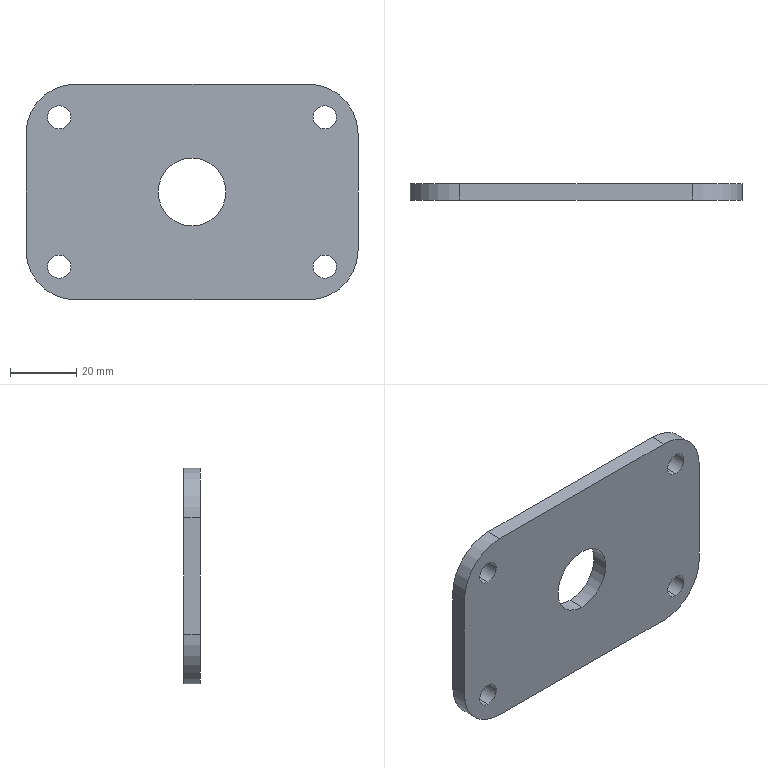Part | SolidWorks | features 3DProfileFeature 2, HoleWzd 2, Extrusion 1, LPattern 1 | 1 solid | 20 faces | box 100 x 5 x 65 mm | volume 29130 mm3 | cylinder 14 | plane 6 | commonest cylinder face diameters 7 x8 30 x4 20.4 x2
STEP:
#1=CARTESIAN_POINT('',(40.,0.,19.));
#2=VERTEX_POINT('',#1);
#3=CARTESIAN_POINT('',(40.,0.,26.));
#4=VERTEX_POINT('',#3);
#5=CARTESIAN_POINT('',(40.,0.,22.5));
#6=DIRECTION('',(0.,1.,0.));
#7=DIRECTION('',(0.,0.,1.));
#8=AXIS2_PLACEMENT_3D('',#5,#6,#7);
#9=CIRCLE('',#8,3.5);
#10=EDGE_CURVE('',#2,#4,#9,.T.);
#11=ORIENTED_EDGE('',*,*,#10,.F.);
#12=CARTESIAN_POINT('',(40.,5.,19.));
#13=VERTEX_POINT('',#12);
#14=CARTESIAN_POINT('',(40.,5.,19.));
#15=DIRECTION('',(0.,1.,0.));
#16=VECTOR('',#15,1000.);
#17=LINE('',#14,#16);
#18=EDGE_CURVE('',#2,#13,#17,.T.);
#19=ORIENTED_EDGE('',*,*,#18,.T.);
#20=CARTESIAN_POINT('',(40.,5.,26.));
#21=VERTEX_POINT('',#20);
#22=CARTESIAN_POINT('',(40.,5.,22.5));
#23=DIRECTION('',(0.,1.,0.));
#24=DIRECTION('',(0.,0.,1.));
#25=AXIS2_PLACEMENT_3D('',#22,#23,#24);
#26=CIRCLE('',#25,3.5);
#27=EDGE_CURVE('',#13,#21,#26,.T.);
#28=ORIENTED_EDGE('',*,*,#27,.T.);
#29=CARTESIAN_POINT('',(40.,5.,26.));
#30=DIRECTION('',(0.,1.,0.));
#31=VECTOR('',#30,1000.);
#32=LINE('',#29,#31);
#33=EDGE_CURVE('',#4,#21,#32,.T.);
#34=ORIENTED_EDGE('',*,*,#33,.F.);
#35=EDGE_LOOP('',(#11,#19,#28,#34));
#36=FACE_OUTER_BOUND('',#35,.T.);
#37=CARTESIAN_POINT('',(40.,5.,22.5));
#38=DIRECTION('',(0.,1.,0.));
#39=DIRECTION('',(0.,0.,1.));
#40=AXIS2_PLACEMENT_3D('',#37,#38,#39);
#41=CYLINDRICAL_SURFACE('',#40,3.5);
#42=ADVANCED_FACE('',(#36),#41,.F.);
#43=CARTESIAN_POINT('',(40.,0.,-26.));
#44=VERTEX_POINT('',#43);
#45=CARTESIAN_POINT('',(40.,0.,-19.));
#46=VERTEX_POINT('',#45);
#47=CARTESIAN_POINT('',(40.,0.,-22.5));
#48=DIRECTION('',(0.,1.,0.));
#49=DIRECTION('',(0.,0.,1.));
#50=AXIS2_PLACEMENT_3D('',#47,#48,#49);
#51=CIRCLE('',#50,3.5);
#52=EDGE_CURVE('',#44,#46,#51,.T.);
#53=ORIENTED_EDGE('',*,*,#52,.F.);
#54=CARTESIAN_POINT('',(40.,5.,-26.));
#55=VERTEX_POINT('',#54);
#56=CARTESIAN_POINT('',(40.,5.,-26.));
#57=DIRECTION('',(0.,1.,0.));
#58=VECTOR('',#57,1000.);
#59=LINE('',#56,#58);
#60=EDGE_CURVE('',#44,#55,#59,.T.);
#61=ORIENTED_EDGE('',*,*,#60,.T.);
#62=CARTESIAN_POINT('',(40.,5.,-19.));
#63=VERTEX_POINT('',#62);
#64=CARTESIAN_POINT('',(40.,5.,-22.5));
#65=DIRECTION('',(0.,1.,0.));
#66=DIRECTION('',(0.,0.,1.));
#67=AXIS2_PLACEMENT_3D('',#64,#65,#66);
#68=CIRCLE('',#67,3.5);
#69=EDGE_CURVE('',#55,#63,#68,.T.);
#70=ORIENTED_EDGE('',*,*,#69,.T.);
#71=CARTESIAN_POINT('',(40.,5.,-19.));
#72=DIRECTION('',(0.,1.,0.));
#73=VECTOR('',#72,1000.);
#74=LINE('',#71,#73);
#75=EDGE_CURVE('',#46,#63,#74,.T.);
#76=ORIENTED_EDGE('',*,*,#75,.F.);
#77=EDGE_LOOP('',(#53,#61,#70,#76));
#78=FACE_OUTER_BOUND('',#77,.T.);
#79=CARTESIAN_POINT('',(40.,5.,-22.5));
#80=DIRECTION('',(0.,1.,0.));
#81=DIRECTION('',(0.,0.,1.));
#82=AXIS2_PLACEMENT_3D('',#79,#80,#81);
#83=CYLINDRICAL_SURFACE('',#82,3.5);
#84=ADVANCED_FACE('',(#78),#83,.F.);
#85=CARTESIAN_POINT('',(-40.,0.,19.));
#86=VERTEX_POINT('',#85);
#87=CARTESIAN_POINT('',(-40.,0.,26.));
#88=VERTEX_POINT('',#87);
#89=CARTESIAN_POINT('',(-40.,0.,22.5));
#90=DIRECTION('',(0.,1.,0.));
#91=DIRECTION('',(0.,0.,1.));
#92=AXIS2_PLACEMENT_3D('',#89,#90,#91);
#93=CIRCLE('',#92,3.5);
#94=EDGE_CURVE('',#86,#88,#93,.T.);
#95=ORIENTED_EDGE('',*,*,#94,.F.);
#96=CARTESIAN_POINT('',(-40.,5.,19.));
#97=VERTEX_POINT('',#96);
#98=CARTESIAN_POINT('',(-40.,5.,19.));
#99=DIRECTION('',(0.,1.,0.));
#100=VECTOR('',#99,1000.);
#101=LINE('',#98,#100);
#102=EDGE_CURVE('',#86,#97,#101,.T.);
#103=ORIENTED_EDGE('',*,*,#102,.T.);
#104=CARTESIAN_POINT('',(-40.,5.,26.));
#105=VERTEX_POINT('',#104);
#106=CARTESIAN_POINT('',(-40.,5.,22.5));
#107=DIRECTION('',(0.,1.,0.));
#108=DIRECTION('',(0.,0.,1.));
#109=AXIS2_PLACEMENT_3D('',#106,#107,#108);
#110=CIRCLE('',#109,3.5);
#111=EDGE_CURVE('',#97,#105,#110,.T.);
#112=ORIENTED_EDGE('',*,*,#111,.T.);
#113=CARTESIAN_POINT('',(-40.,5.,26.));
#114=DIRECTION('',(0.,1.,0.));
#115=VECTOR('',#114,1000.);
#116=LINE('',#113,#115);
#117=EDGE_CURVE('',#88,#105,#116,.T.);
#118=ORIENTED_EDGE('',*,*,#117,.F.);
#119=EDGE_LOOP('',(#95,#103,#112,#118));
#120=FACE_OUTER_BOUND('',#119,.T.);
#121=CARTESIAN_POINT('',(-40.,5.,22.5));
#122=DIRECTION('',(0.,1.,0.));
#123=DIRECTION('',(0.,0.,1.));
#124=AXIS2_PLACEMENT_3D('',#121,#122,#123);
#125=CYLINDRICAL_SURFACE('',#124,3.5);
#126=ADVANCED_FACE('',(#120),#125,.F.);
#127=CARTESIAN_POINT('',(-40.,0.,-26.));
#128=VERTEX_POINT('',#127);
#129=CARTESIAN_POINT('',(-40.,0.,-19.));
#130=VERTEX_POINT('',#129);
#131=CARTESIAN_POINT('',(-40.,0.,-22.5));
#132=DIRECTION('',(0.,1.,0.));
#133=DIRECTION('',(0.,0.,1.));
#134=AXIS2_PLACEMENT_3D('',#131,#132,#133);
#135=CIRCLE('',#134,3.5);
#136=EDGE_CURVE('',#128,#130,#135,.T.);
#137=ORIENTED_EDGE('',*,*,#136,.F.);
#138=CARTESIAN_POINT('',(-40.,5.,-26.));
#139=VERTEX_POINT('',#138);
#140=CARTESIAN_POINT('',(-40.,5.,-26.));
#141=DIRECTION('',(0.,1.,0.));
#142=VECTOR('',#141,1000.);
#143=LINE('',#140,#142);
#144=EDGE_CURVE('',#128,#139,#143,.T.);
#145=ORIENTED_EDGE('',*,*,#144,.T.);
#146=CARTESIAN_POINT('',(-40.,5.,-19.));
#147=VERTEX_POINT('',#146);
#148=CARTESIAN_POINT('',(-40.,5.,-22.5));
#149=DIRECTION('',(0.,1.,0.));
#150=DIRECTION('',(0.,0.,1.));
#151=AXIS2_PLACEMENT_3D('',#148,#149,#150);
#152=CIRCLE('',#151,3.5);
#153=EDGE_CURVE('',#139,#147,#152,.T.);
#154=ORIENTED_EDGE('',*,*,#153,.T.);
#155=CARTESIAN_POINT('',(-40.,5.,-19.));
#156=DIRECTION('',(0.,1.,0.));
#157=VECTOR('',#156,1000.);
#158=LINE('',#155,#157);
#159=EDGE_CURVE('',#130,#147,#158,.T.);
#160=ORIENTED_EDGE('',*,*,#159,.F.);
#161=EDGE_LOOP('',(#137,#145,#154,#160));
#162=FACE_OUTER_BOUND('',#161,.T.);
#163=CARTESIAN_POINT('',(-40.,5.,-22.5));
#164=DIRECTION('',(0.,1.,0.));
#165=DIRECTION('',(0.,0.,1.));
#166=AXIS2_PLACEMENT_3D('',#163,#164,#165);
#167=CYLINDRICAL_SURFACE('',#166,3.5);
#168=ADVANCED_FACE('',(#162),#167,.F.);
#169=CARTESIAN_POINT('',(0.,0.,-10.2));
#170=VERTEX_POINT('',#169);
#171=CARTESIAN_POINT('',(0.,0.,10.2));
#172=VERTEX_POINT('',#171);
#173=CARTESIAN_POINT('',(0.,0.,0.));
#174=DIRECTION('',(0.,1.,0.));
#175=DIRECTION('',(0.,0.,1.));
#176=AXIS2_PLACEMENT_3D('',#173,#174,#175);
#177=CIRCLE('',#176,10.2);
#178=EDGE_CURVE('',#170,#172,#177,.T.);
#179=ORIENTED_EDGE('',*,*,#178,.F.);
#180=CARTESIAN_POINT('',(0.,5.,-10.2));
#181=VERTEX_POINT('',#180);
#182=CARTESIAN_POINT('',(0.,5.,-10.2));
#183=DIRECTION('',(0.,1.,0.));
#184=VECTOR('',#183,1000.);
#185=LINE('',#182,#184);
#186=EDGE_CURVE('',#170,#181,#185,.T.);
#187=ORIENTED_EDGE('',*,*,#186,.T.);
#188=CARTESIAN_POINT('',(0.,5.,10.2));
#189=VERTEX_POINT('',#188);
#190=CARTESIAN_POINT('',(0.,5.,0.));
#191=DIRECTION('',(0.,1.,0.));
#192=DIRECTION('',(0.,0.,1.));
#193=AXIS2_PLACEMENT_3D('',#190,#191,#192);
#194=CIRCLE('',#193,10.2);
#195=EDGE_CURVE('',#181,#189,#194,.T.);
#196=ORIENTED_EDGE('',*,*,#195,.T.);
#197=CARTESIAN_POINT('',(0.,5.,10.2));
#198=DIRECTION('',(0.,1.,0.));
#199=VECTOR('',#198,1000.);
#200=LINE('',#197,#199);
#201=EDGE_CURVE('',#172,#189,#200,.T.);
#202=ORIENTED_EDGE('',*,*,#201,.F.);
#203=EDGE_LOOP('',(#179,#187,#196,#202));
#204=FACE_OUTER_BOUND('',#203,.T.);
#205=CARTESIAN_POINT('',(0.,5.,0.));
#206=DIRECTION('',(0.,1.,0.));
#207=DIRECTION('',(0.,0.,1.));
#208=AXIS2_PLACEMENT_3D('',#205,#206,#207);
#209=CYLINDRICAL_SURFACE('',#208,10.2);
#210=ADVANCED_FACE('',(#204),#209,.F.);
#211=CARTESIAN_POINT('',(-40.,0.,22.5));
#212=DIRECTION('',(0.,1.,0.));
#213=DIRECTION('',(0.,0.,1.));
#214=AXIS2_PLACEMENT_3D('',#211,#212,#213);
#215=CIRCLE('',#214,3.5);
#216=EDGE_CURVE('',#88,#86,#215,.T.);
#217=ORIENTED_EDGE('',*,*,#216,.T.);
#218=ORIENTED_EDGE('',*,*,#94,.T.);
#219=EDGE_LOOP('',(#217,#218));
#220=FACE_BOUND('',#219,.T.);
#221=CARTESIAN_POINT('',(-40.,0.,-22.5));
#222=DIRECTION('',(0.,1.,0.));
#223=DIRECTION('',(0.,0.,1.));
#224=AXIS2_PLACEMENT_3D('',#221,#222,#223);
#225=CIRCLE('',#224,3.5);
#226=EDGE_CURVE('',#130,#128,#225,.T.);
#227=ORIENTED_EDGE('',*,*,#226,.T.);
#228=ORIENTED_EDGE('',*,*,#136,.T.);
#229=EDGE_LOOP('',(#227,#228));
#230=FACE_BOUND('',#229,.T.);
#231=CARTESIAN_POINT('',(0.,0.,0.));
#232=DIRECTION('',(0.,1.,0.));
#233=DIRECTION('',(0.,0.,1.));
#234=AXIS2_PLACEMENT_3D('',#231,#232,#233);
#235=CIRCLE('',#234,10.2);
#236=EDGE_CURVE('',#172,#170,#235,.T.);
#237=ORIENTED_EDGE('',*,*,#236,.T.);
#238=ORIENTED_EDGE('',*,*,#178,.T.);
#239=EDGE_LOOP('',(#237,#238));
#240=FACE_BOUND('',#239,.T.);
#241=CARTESIAN_POINT('',(50.,0.,-17.5));
#242=VERTEX_POINT('',#241);
#243=CARTESIAN_POINT('',(35.,0.,-32.5));
#244=VERTEX_POINT('',#243);
#245=CARTESIAN_POINT('',(35.,0.,-17.5));
#246=DIRECTION('',(0.,1.,0.));
#247=DIRECTION('',(0.,0.,-1.));
#248=AXIS2_PLACEMENT_3D('',#245,#246,#247);
#249=CIRCLE('',#248,15.);
#250=EDGE_CURVE('',#242,#244,#249,.T.);
#251=ORIENTED_EDGE('',*,*,#250,.F.);
#252=CARTESIAN_POINT('',(50.,0.,17.5));
#253=VERTEX_POINT('',#252);
#254=CARTESIAN_POINT('',(50.,0.,-17.5));
#255=DIRECTION('',(0.,0.,-1.));
#256=VECTOR('',#255,1000.);
#257=LINE('',#254,#256);
#258=EDGE_CURVE('',#253,#242,#257,.T.);
#259=ORIENTED_EDGE('',*,*,#258,.F.);
#260=CARTESIAN_POINT('',(35.,0.,32.5));
#261=VERTEX_POINT('',#260);
#262=CARTESIAN_POINT('',(35.,0.,17.5));
#263=DIRECTION('',(0.,1.,0.));
#264=DIRECTION('',(0.,0.,1.));
#265=AXIS2_PLACEMENT_3D('',#262,#263,#264);
#266=CIRCLE('',#265,15.);
#267=EDGE_CURVE('',#261,#253,#266,.T.);
#268=ORIENTED_EDGE('',*,*,#267,.F.);
#269=CARTESIAN_POINT('',(-35.,0.,32.5));
#270=VERTEX_POINT('',#269);
#271=CARTESIAN_POINT('',(-35.,0.,32.5));
#272=DIRECTION('',(1.,0.,0.));
#273=VECTOR('',#272,1000.);
#274=LINE('',#271,#273);
#275=EDGE_CURVE('',#270,#261,#274,.T.);
#276=ORIENTED_EDGE('',*,*,#275,.F.);
#277=CARTESIAN_POINT('',(-50.,0.,17.5));
#278=VERTEX_POINT('',#277);
#279=CARTESIAN_POINT('',(-35.,0.,17.5));
#280=DIRECTION('',(0.,1.,0.));
#281=DIRECTION('',(0.,0.,1.));
#282=AXIS2_PLACEMENT_3D('',#279,#280,#281);
#283=CIRCLE('',#282,15.);
#284=EDGE_CURVE('',#278,#270,#283,.T.);
#285=ORIENTED_EDGE('',*,*,#284,.F.);
#286=CARTESIAN_POINT('',(-50.,0.,-17.5));
#287=VERTEX_POINT('',#286);
#288=CARTESIAN_POINT('',(-50.,0.,-17.5));
#289=DIRECTION('',(0.,0.,1.));
#290=VECTOR('',#289,1000.);
#291=LINE('',#288,#290);
#292=EDGE_CURVE('',#287,#278,#291,.T.);
#293=ORIENTED_EDGE('',*,*,#292,.F.);
#294=CARTESIAN_POINT('',(-35.,0.,-32.5));
#295=VERTEX_POINT('',#294);
#296=CARTESIAN_POINT('',(-35.,0.,-17.5));
#297=DIRECTION('',(0.,1.,0.));
#298=DIRECTION('',(0.,0.,1.));
#299=AXIS2_PLACEMENT_3D('',#296,#297,#298);
#300=CIRCLE('',#299,15.);
#301=EDGE_CURVE('',#295,#287,#300,.T.);
#302=ORIENTED_EDGE('',*,*,#301,.F.);
#303=CARTESIAN_POINT('',(-35.,0.,-32.5));
#304=DIRECTION('',(-1.,0.,0.));
#305=VECTOR('',#304,1000.);
#306=LINE('',#303,#305);
#307=EDGE_CURVE('',#244,#295,#306,.T.);
#308=ORIENTED_EDGE('',*,*,#307,.F.);
#309=EDGE_LOOP('',(#251,#259,#268,#276,#285,#293,#302,#308));
#310=FACE_OUTER_BOUND('',#309,.T.);
#311=CARTESIAN_POINT('',(40.,0.,-22.5));
#312=DIRECTION('',(0.,1.,0.));
#313=DIRECTION('',(0.,0.,1.));
#314=AXIS2_PLACEMENT_3D('',#311,#312,#313);
#315=CIRCLE('',#314,3.5);
#316=EDGE_CURVE('',#46,#44,#315,.T.);
#317=ORIENTED_EDGE('',*,*,#316,.T.);
#318=ORIENTED_EDGE('',*,*,#52,.T.);
#319=EDGE_LOOP('',(#317,#318));
#320=FACE_BOUND('',#319,.T.);
#321=CARTESIAN_POINT('',(40.,0.,22.5));
#322=DIRECTION('',(0.,1.,0.));
#323=DIRECTION('',(0.,0.,1.));
#324=AXIS2_PLACEMENT_3D('',#321,#322,#323);
#325=CIRCLE('',#324,3.5);
#326=EDGE_CURVE('',#4,#2,#325,.T.);
#327=ORIENTED_EDGE('',*,*,#326,.T.);
#328=ORIENTED_EDGE('',*,*,#10,.T.);
#329=EDGE_LOOP('',(#327,#328));
#330=FACE_BOUND('',#329,.T.);
#331=CARTESIAN_POINT('',(35.,0.,-17.5));
#332=DIRECTION('',(0.,-1.,0.));
#333=DIRECTION('',(0.,0.,-1.));
#334=AXIS2_PLACEMENT_3D('',#331,#332,#333);
#335=PLANE('',#334);
#336=ADVANCED_FACE('',(#220,#230,#240,#310,#320,#330),#335,.T.);
#337=CARTESIAN_POINT('',(40.,5.,22.5));
#338=DIRECTION('',(0.,1.,0.));
#339=DIRECTION('',(0.,0.,1.));
#340=AXIS2_PLACEMENT_3D('',#337,#338,#339);
#341=CIRCLE('',#340,3.5);
#342=EDGE_CURVE('',#21,#13,#341,.T.);
#343=ORIENTED_EDGE('',*,*,#342,.F.);
#344=ORIENTED_EDGE('',*,*,#27,.F.);
#345=EDGE_LOOP('',(#343,#344));
#346=FACE_BOUND('',#345,.T.);
#347=CARTESIAN_POINT('',(-40.,5.,-22.5));
#348=DIRECTION('',(0.,1.,0.));
#349=DIRECTION('',(0.,0.,1.));
#350=AXIS2_PLACEMENT_3D('',#347,#348,#349);
#351=CIRCLE('',#350,3.5);
#352=EDGE_CURVE('',#147,#139,#351,.T.);
#353=ORIENTED_EDGE('',*,*,#352,.F.);
#354=ORIENTED_EDGE('',*,*,#153,.F.);
#355=EDGE_LOOP('',(#353,#354));
#356=FACE_BOUND('',#355,.T.);
#357=CARTESIAN_POINT('',(50.,5.,-17.5));
#358=VERTEX_POINT('',#357);
#359=CARTESIAN_POINT('',(35.,5.,-32.5));
#360=VERTEX_POINT('',#359);
#361=CARTESIAN_POINT('',(35.,5.,-17.5));
#362=DIRECTION('',(0.,1.,0.));
#363=DIRECTION('',(0.,0.,-1.));
#364=AXIS2_PLACEMENT_3D('',#361,#362,#363);
#365=CIRCLE('',#364,15.);
#366=EDGE_CURVE('',#358,#360,#365,.T.);
#367=ORIENTED_EDGE('',*,*,#366,.T.);
#368=CARTESIAN_POINT('',(-35.,5.,-32.5));
#369=VERTEX_POINT('',#368);
#370=CARTESIAN_POINT('',(-35.,5.,-32.5));
#371=DIRECTION('',(-1.,0.,0.));
#372=VECTOR('',#371,1000.);
#373=LINE('',#370,#372);
#374=EDGE_CURVE('',#360,#369,#373,.T.);
#375=ORIENTED_EDGE('',*,*,#374,.T.);
#376=CARTESIAN_POINT('',(-50.,5.,-17.5));
#377=VERTEX_POINT('',#376);
#378=CARTESIAN_POINT('',(-35.,5.,-17.5));
#379=DIRECTION('',(0.,1.,0.));
#380=DIRECTION('',(0.,0.,1.));
#381=AXIS2_PLACEMENT_3D('',#378,#379,#380);
#382=CIRCLE('',#381,15.);
#383=EDGE_CURVE('',#369,#377,#382,.T.);
#384=ORIENTED_EDGE('',*,*,#383,.T.);
#385=CARTESIAN_POINT('',(-50.,5.,17.5));
#386=VERTEX_POINT('',#385);
#387=CARTESIAN_POINT('',(-50.,5.,-17.5));
#388=DIRECTION('',(0.,0.,1.));
#389=VECTOR('',#388,1000.);
#390=LINE('',#387,#389);
#391=EDGE_CURVE('',#377,#386,#390,.T.);
#392=ORIENTED_EDGE('',*,*,#391,.T.);
#393=CARTESIAN_POINT('',(-35.,5.,32.5));
#394=VERTEX_POINT('',#393);
#395=CARTESIAN_POINT('',(-35.,5.,17.5));
#396=DIRECTION('',(0.,1.,0.));
#397=DIRECTION('',(0.,0.,1.));
#398=AXIS2_PLACEMENT_3D('',#395,#396,#397);
#399=CIRCLE('',#398,15.);
#400=EDGE_CURVE('',#386,#394,#399,.T.);
#401=ORIENTED_EDGE('',*,*,#400,.T.);
#402=CARTESIAN_POINT('',(35.,5.,32.5));
#403=VERTEX_POINT('',#402);
#404=CARTESIAN_POINT('',(-35.,5.,32.5));
#405=DIRECTION('',(1.,0.,0.));
#406=VECTOR('',#405,1000.);
#407=LINE('',#404,#406);
#408=EDGE_CURVE('',#394,#403,#407,.T.);
#409=ORIENTED_EDGE('',*,*,#408,.T.);
#410=CARTESIAN_POINT('',(50.,5.,17.5));
#411=VERTEX_POINT('',#410);
#412=CARTESIAN_POINT('',(35.,5.,17.5));
#413=DIRECTION('',(0.,1.,0.));
#414=DIRECTION('',(0.,0.,1.));
#415=AXIS2_PLACEMENT_3D('',#412,#413,#414);
#416=CIRCLE('',#415,15.);
#417=EDGE_CURVE('',#403,#411,#416,.T.);
#418=ORIENTED_EDGE('',*,*,#417,.T.);
#419=CARTESIAN_POINT('',(50.,5.,-17.5));
#420=DIRECTION('',(0.,0.,-1.));
#421=VECTOR('',#420,1000.);
#422=LINE('',#419,#421);
#423=EDGE_CURVE('',#411,#358,#422,.T.);
#424=ORIENTED_EDGE('',*,*,#423,.T.);
#425=EDGE_LOOP('',(#367,#375,#384,#392,#401,#409,#418,#424));
#426=FACE_OUTER_BOUND('',#425,.T.);
#427=CARTESIAN_POINT('',(0.,5.,0.));
#428=DIRECTION('',(0.,1.,0.));
#429=DIRECTION('',(0.,0.,1.));
#430=AXIS2_PLACEMENT_3D('',#427,#428,#429);
#431=CIRCLE('',#430,10.2);
#432=EDGE_CURVE('',#189,#181,#431,.T.);
#433=ORIENTED_EDGE('',*,*,#432,.F.);
#434=ORIENTED_EDGE('',*,*,#195,.F.);
#435=EDGE_LOOP('',(#433,#434));
#436=FACE_BOUND('',#435,.T.);
#437=CARTESIAN_POINT('',(-40.,5.,22.5));
#438=DIRECTION('',(0.,1.,0.));
#439=DIRECTION('',(0.,0.,1.));
#440=AXIS2_PLACEMENT_3D('',#437,#438,#439);
#441=CIRCLE('',#440,3.5);
#442=EDGE_CURVE('',#105,#97,#441,.T.);
#443=ORIENTED_EDGE('',*,*,#442,.F.);
#444=ORIENTED_EDGE('',*,*,#111,.F.);
#445=EDGE_LOOP('',(#443,#444));
#446=FACE_BOUND('',#445,.T.);
#447=CARTESIAN_POINT('',(40.,5.,-22.5));
#448=DIRECTION('',(0.,1.,0.));
#449=DIRECTION('',(0.,0.,1.));
#450=AXIS2_PLACEMENT_3D('',#447,#448,#449);
#451=CIRCLE('',#450,3.5);
#452=EDGE_CURVE('',#63,#55,#451,.T.);
#453=ORIENTED_EDGE('',*,*,#452,.F.);
#454=ORIENTED_EDGE('',*,*,#69,.F.);
#455=EDGE_LOOP('',(#453,#454));
#456=FACE_BOUND('',#455,.T.);
#457=CARTESIAN_POINT('',(35.,5.,-17.5));
#458=DIRECTION('',(0.,-1.,0.));
#459=DIRECTION('',(0.,0.,-1.));
#460=AXIS2_PLACEMENT_3D('',#457,#458,#459);
#461=PLANE('',#460);
#462=ADVANCED_FACE('',(#346,#356,#426,#436,#446,#456),#461,.F.);
#463=ORIENTED_EDGE('',*,*,#250,.T.);
#464=CARTESIAN_POINT('',(35.,5.,-32.5));
#465=DIRECTION('',(0.,-1.,0.));
#466=VECTOR('',#465,1000.);
#467=LINE('',#464,#466);
#468=EDGE_CURVE('',#360,#244,#467,.T.);
#469=ORIENTED_EDGE('',*,*,#468,.F.);
#470=ORIENTED_EDGE('',*,*,#366,.F.);
#471=CARTESIAN_POINT('',(50.,5.,-17.5));
#472=DIRECTION('',(0.,-1.,0.));
#473=VECTOR('',#472,1000.);
#474=LINE('',#471,#473);
#475=EDGE_CURVE('',#358,#242,#474,.T.);
#476=ORIENTED_EDGE('',*,*,#475,.T.);
#477=EDGE_LOOP('',(#463,#469,#470,#476));
#478=FACE_OUTER_BOUND('',#477,.T.);
#479=CARTESIAN_POINT('',(35.,5.,-17.5));
#480=DIRECTION('',(0.,-1.,0.));
#481=DIRECTION('',(0.,0.,-1.));
#482=AXIS2_PLACEMENT_3D('',#479,#480,#481);
#483=CYLINDRICAL_SURFACE('',#482,15.);
#484=ADVANCED_FACE('',(#478),#483,.T.);
#485=ORIENTED_EDGE('',*,*,#307,.T.);
#486=CARTESIAN_POINT('',(-35.,5.,-32.5));
#487=DIRECTION('',(0.,-1.,0.));
#488=VECTOR('',#487,1000.);
#489=LINE('',#486,#488);
#490=EDGE_CURVE('',#369,#295,#489,.T.);
#491=ORIENTED_EDGE('',*,*,#490,.F.);
#492=ORIENTED_EDGE('',*,*,#374,.F.);
#493=ORIENTED_EDGE('',*,*,#468,.T.);
#494=EDGE_LOOP('',(#485,#491,#492,#493));
#495=FACE_OUTER_BOUND('',#494,.T.);
#496=CARTESIAN_POINT('',(-35.,5.,-32.5));
#497=DIRECTION('',(0.,0.,1.));
#498=DIRECTION('',(1.,0.,0.));
#499=AXIS2_PLACEMENT_3D('',#496,#497,#498);
#500=PLANE('',#499);
#501=ADVANCED_FACE('',(#495),#500,.F.);
#502=ORIENTED_EDGE('',*,*,#301,.T.);
#503=CARTESIAN_POINT('',(-50.,5.,-17.5));
#504=DIRECTION('',(0.,-1.,0.));
#505=VECTOR('',#504,1000.);
#506=LINE('',#503,#505);
#507=EDGE_CURVE('',#377,#287,#506,.T.);
#508=ORIENTED_EDGE('',*,*,#507,.F.);
#509=ORIENTED_EDGE('',*,*,#383,.F.);
#510=ORIENTED_EDGE('',*,*,#490,.T.);
#511=EDGE_LOOP('',(#502,#508,#509,#510));
#512=FACE_OUTER_BOUND('',#511,.T.);
#513=CARTESIAN_POINT('',(-35.,5.,-17.5));
#514=DIRECTION('',(0.,-1.,0.));
#515=DIRECTION('',(0.,0.,-1.));
#516=AXIS2_PLACEMENT_3D('',#513,#514,#515);
#517=CYLINDRICAL_SURFACE('',#516,15.);
#518=ADVANCED_FACE('',(#512),#517,.T.);
#519=ORIENTED_EDGE('',*,*,#292,.T.);
#520=CARTESIAN_POINT('',(-50.,5.,17.5));
#521=DIRECTION('',(0.,-1.,0.));
#522=VECTOR('',#521,1000.);
#523=LINE('',#520,#522);
#524=EDGE_CURVE('',#386,#278,#523,.T.);
#525=ORIENTED_EDGE('',*,*,#524,.F.);
#526=ORIENTED_EDGE('',*,*,#391,.F.);
#527=ORIENTED_EDGE('',*,*,#507,.T.);
#528=EDGE_LOOP('',(#519,#525,#526,#527));
#529=FACE_OUTER_BOUND('',#528,.T.);
#530=CARTESIAN_POINT('',(-50.,5.,-17.5));
#531=DIRECTION('',(1.,0.,0.));
#532=DIRECTION('',(0.,0.,-1.));
#533=AXIS2_PLACEMENT_3D('',#530,#531,#532);
#534=PLANE('',#533);
#535=ADVANCED_FACE('',(#529),#534,.F.);
#536=ORIENTED_EDGE('',*,*,#284,.T.);
#537=CARTESIAN_POINT('',(-35.,5.,32.5));
#538=DIRECTION('',(0.,-1.,0.));
#539=VECTOR('',#538,1000.);
#540=LINE('',#537,#539);
#541=EDGE_CURVE('',#394,#270,#540,.T.);
#542=ORIENTED_EDGE('',*,*,#541,.F.);
#543=ORIENTED_EDGE('',*,*,#400,.F.);
#544=ORIENTED_EDGE('',*,*,#524,.T.);
#545=EDGE_LOOP('',(#536,#542,#543,#544));
#546=FACE_OUTER_BOUND('',#545,.T.);
#547=CARTESIAN_POINT('',(-35.,5.,17.5));
#548=DIRECTION('',(0.,-1.,0.));
#549=DIRECTION('',(0.,0.,-1.));
#550=AXIS2_PLACEMENT_3D('',#547,#548,#549);
#551=CYLINDRICAL_SURFACE('',#550,15.);
#552=ADVANCED_FACE('',(#546),#551,.T.);
#553=ORIENTED_EDGE('',*,*,#275,.T.);
#554=CARTESIAN_POINT('',(35.,5.,32.5));
#555=DIRECTION('',(0.,-1.,0.));
#556=VECTOR('',#555,1000.);
#557=LINE('',#554,#556);
#558=EDGE_CURVE('',#403,#261,#557,.T.);
#559=ORIENTED_EDGE('',*,*,#558,.F.);
#560=ORIENTED_EDGE('',*,*,#408,.F.);
#561=ORIENTED_EDGE('',*,*,#541,.T.);
#562=EDGE_LOOP('',(#553,#559,#560,#561));
#563=FACE_OUTER_BOUND('',#562,.T.);
#564=CARTESIAN_POINT('',(-35.,5.,32.5));
#565=DIRECTION('',(0.,0.,-1.));
#566=DIRECTION('',(-1.,0.,0.));
#567=AXIS2_PLACEMENT_3D('',#564,#565,#566);
#568=PLANE('',#567);
#569=ADVANCED_FACE('',(#563),#568,.F.);
#570=ORIENTED_EDGE('',*,*,#267,.T.);
#571=CARTESIAN_POINT('',(50.,5.,17.5));
#572=DIRECTION('',(0.,-1.,0.));
#573=VECTOR('',#572,1000.);
#574=LINE('',#571,#573);
#575=EDGE_CURVE('',#411,#253,#574,.T.);
#576=ORIENTED_EDGE('',*,*,#575,.F.);
#577=ORIENTED_EDGE('',*,*,#417,.F.);
#578=ORIENTED_EDGE('',*,*,#558,.T.);
#579=EDGE_LOOP('',(#570,#576,#577,#578));
#580=FACE_OUTER_BOUND('',#579,.T.);
#581=CARTESIAN_POINT('',(35.,5.,17.5));
#582=DIRECTION('',(0.,-1.,0.));
#583=DIRECTION('',(0.,0.,-1.));
#584=AXIS2_PLACEMENT_3D('',#581,#582,#583);
#585=CYLINDRICAL_SURFACE('',#584,15.);
#586=ADVANCED_FACE('',(#580),#585,.T.);
#587=ORIENTED_EDGE('',*,*,#258,.T.);
#588=ORIENTED_EDGE('',*,*,#475,.F.);
#589=ORIENTED_EDGE('',*,*,#423,.F.);
#590=ORIENTED_EDGE('',*,*,#575,.T.);
#591=EDGE_LOOP('',(#587,#588,#589,#590));
#592=FACE_OUTER_BOUND('',#591,.T.);
#593=CARTESIAN_POINT('',(50.,5.,-17.5));
#594=DIRECTION('',(-1.,0.,0.));
#595=DIRECTION('',(0.,0.,1.));
#596=AXIS2_PLACEMENT_3D('',#593,#594,#595);
#597=PLANE('',#596);
#598=ADVANCED_FACE('',(#592),#597,.F.);
#599=ORIENTED_EDGE('',*,*,#186,.F.);
#600=ORIENTED_EDGE('',*,*,#236,.F.);
#601=ORIENTED_EDGE('',*,*,#201,.T.);
#602=ORIENTED_EDGE('',*,*,#432,.T.);
#603=EDGE_LOOP('',(#599,#600,#601,#602));
#604=FACE_OUTER_BOUND('',#603,.T.);
#605=CARTESIAN_POINT('',(0.,5.,0.));
#606=DIRECTION('',(0.,1.,0.));
#607=DIRECTION('',(0.,0.,1.));
#608=AXIS2_PLACEMENT_3D('',#605,#606,#607);
#609=CYLINDRICAL_SURFACE('',#608,10.2);
#610=ADVANCED_FACE('',(#604),#609,.F.);
#611=ORIENTED_EDGE('',*,*,#144,.F.);
#612=ORIENTED_EDGE('',*,*,#226,.F.);
#613=ORIENTED_EDGE('',*,*,#159,.T.);
#614=ORIENTED_EDGE('',*,*,#352,.T.);
#615=EDGE_LOOP('',(#611,#612,#613,#614));
#616=FACE_OUTER_BOUND('',#615,.T.);
#617=CARTESIAN_POINT('',(-40.,5.,-22.5));
#618=DIRECTION('',(0.,1.,0.));
#619=DIRECTION('',(0.,0.,1.));
#620=AXIS2_PLACEMENT_3D('',#617,#618,#619);
#621=CYLINDRICAL_SURFACE('',#620,3.5);
#622=ADVANCED_FACE('',(#616),#621,.F.);
#623=ORIENTED_EDGE('',*,*,#102,.F.);
#624=ORIENTED_EDGE('',*,*,#216,.F.);
#625=ORIENTED_EDGE('',*,*,#117,.T.);
#626=ORIENTED_EDGE('',*,*,#442,.T.);
#627=EDGE_LOOP('',(#623,#624,#625,#626));
#628=FACE_OUTER_BOUND('',#627,.T.);
#629=CARTESIAN_POINT('',(-40.,5.,22.5));
#630=DIRECTION('',(0.,1.,0.));
#631=DIRECTION('',(0.,0.,1.));
#632=AXIS2_PLACEMENT_3D('',#629,#630,#631);
#633=CYLINDRICAL_SURFACE('',#632,3.5);
#634=ADVANCED_FACE('',(#628),#633,.F.);
#635=ORIENTED_EDGE('',*,*,#60,.F.);
#636=ORIENTED_EDGE('',*,*,#316,.F.);
#637=ORIENTED_EDGE('',*,*,#75,.T.);
#638=ORIENTED_EDGE('',*,*,#452,.T.);
#639=EDGE_LOOP('',(#635,#636,#637,#638));
#640=FACE_OUTER_BOUND('',#639,.T.);
#641=CARTESIAN_POINT('',(40.,5.,-22.5));
#642=DIRECTION('',(0.,1.,0.));
#643=DIRECTION('',(0.,0.,1.));
#644=AXIS2_PLACEMENT_3D('',#641,#642,#643);
#645=CYLINDRICAL_SURFACE('',#644,3.5);
#646=ADVANCED_FACE('',(#640),#645,.F.);
#647=ORIENTED_EDGE('',*,*,#18,.F.);
#648=ORIENTED_EDGE('',*,*,#326,.F.);
#649=ORIENTED_EDGE('',*,*,#33,.T.);
#650=ORIENTED_EDGE('',*,*,#342,.T.);
#651=EDGE_LOOP('',(#647,#648,#649,#650));
#652=FACE_OUTER_BOUND('',#651,.T.);
#653=CARTESIAN_POINT('',(40.,5.,22.5));
#654=DIRECTION('',(0.,1.,0.));
#655=DIRECTION('',(0.,0.,1.));
#656=AXIS2_PLACEMENT_3D('',#653,#654,#655);
#657=CYLINDRICAL_SURFACE('',#656,3.5);
#658=ADVANCED_FACE('',(#652),#657,.F.);
#659=CLOSED_SHELL('',(#42,#84,#126,#168,#210,#336,#462,#484,#501,#518,#535,#552,#569,#586,#598,#610,#622,#634,#646,#658));
#660=MANIFOLD_SOLID_BREP('',#659);
#661=CARTESIAN_POINT('',(0.,0.,0.));
#662=DIRECTION('',(0.,0.,1.));
#663=DIRECTION('',(1.,0.,0.));
#664=AXIS2_PLACEMENT_3D('',#661,#662,#663);
#665=(LENGTH_UNIT()NAMED_UNIT(*)SI_UNIT(.MILLI.,.METRE.));
#666=UNCERTAINTY_MEASURE_WITH_UNIT(LENGTH_MEASURE(0.00001),#665,'','');
#667=(NAMED_UNIT(*)PLANE_ANGLE_UNIT()SI_UNIT($,.RADIAN.));
#668=(NAMED_UNIT(*)SI_UNIT($,.STERADIAN.)SOLID_ANGLE_UNIT());
#669=(GEOMETRIC_REPRESENTATION_CONTEXT(3)GLOBAL_UNCERTAINTY_ASSIGNED_CONTEXT((#666))GLOBAL_UNIT_ASSIGNED_CONTEXT((#665,#667,#668))REPRESENTATION_CONTEXT('',''));
#670=ADVANCED_BREP_SHAPE_REPRESENTATION('',(#660,#664),#669);